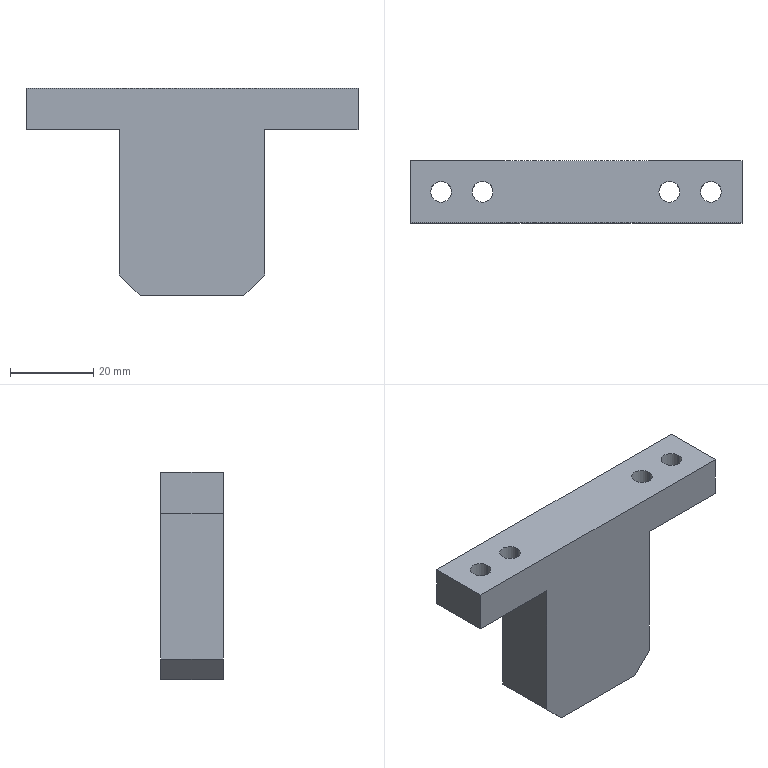Part | SolidWorks | features BaseBody 1 | 1 solid | 20 faces | box 80 x 15 x 50 mm | volume 31840 mm3 | plane 12 | cylinder 8 | commonest cylinder face diameters 5 x8
STEP:
#1=CARTESIAN_POINT('',(10.,7.5,-10.));
#2=VERTEX_POINT('',#1);
#3=CARTESIAN_POINT('',(5.,7.5,-10.));
#4=VERTEX_POINT('',#3);
#5=CARTESIAN_POINT('',(7.5,7.5,-10.));
#6=DIRECTION('',(0.,0.,-1.));
#7=DIRECTION('',(1.,0.,0.));
#8=AXIS2_PLACEMENT_3D('',#5,#6,#7);
#9=CIRCLE('',#8,2.5);
#10=EDGE_CURVE('',#2,#4,#9,.T.);
#11=ORIENTED_EDGE('',*,*,#10,.T.);
#12=CARTESIAN_POINT('',(5.,7.5,0.));
#13=VERTEX_POINT('',#12);
#14=CARTESIAN_POINT('',(5.,7.5,-10.));
#15=DIRECTION('',(0.,0.,1.));
#16=VECTOR('',#15,1000.);
#17=LINE('',#14,#16);
#18=EDGE_CURVE('',#4,#13,#17,.T.);
#19=ORIENTED_EDGE('',*,*,#18,.T.);
#20=CARTESIAN_POINT('',(10.,7.5,0.));
#21=VERTEX_POINT('',#20);
#22=CARTESIAN_POINT('',(7.5,7.5,0.));
#23=DIRECTION('',(0.,0.,1.));
#24=DIRECTION('',(1.,0.,0.));
#25=AXIS2_PLACEMENT_3D('',#22,#23,#24);
#26=CIRCLE('',#25,2.5);
#27=EDGE_CURVE('',#13,#21,#26,.T.);
#28=ORIENTED_EDGE('',*,*,#27,.T.);
#29=CARTESIAN_POINT('',(10.,7.5,-10.));
#30=DIRECTION('',(0.,0.,1.));
#31=VECTOR('',#30,1000.);
#32=LINE('',#29,#31);
#33=EDGE_CURVE('',#2,#21,#32,.T.);
#34=ORIENTED_EDGE('',*,*,#33,.F.);
#35=EDGE_LOOP('',(#11,#19,#28,#34));
#36=FACE_OUTER_BOUND('',#35,.T.);
#37=CARTESIAN_POINT('',(7.5,7.5,-10.));
#38=DIRECTION('',(0.,0.,1.));
#39=DIRECTION('',(1.,0.,0.));
#40=AXIS2_PLACEMENT_3D('',#37,#38,#39);
#41=CYLINDRICAL_SURFACE('',#40,2.5);
#42=ADVANCED_FACE('',(#36),#41,.F.);
#43=CARTESIAN_POINT('',(20.,7.5,-10.));
#44=VERTEX_POINT('',#43);
#45=CARTESIAN_POINT('',(15.,7.5,-10.));
#46=VERTEX_POINT('',#45);
#47=CARTESIAN_POINT('',(17.5,7.5,-10.));
#48=DIRECTION('',(0.,0.,-1.));
#49=DIRECTION('',(1.,0.,0.));
#50=AXIS2_PLACEMENT_3D('',#47,#48,#49);
#51=CIRCLE('',#50,2.5);
#52=EDGE_CURVE('',#44,#46,#51,.T.);
#53=ORIENTED_EDGE('',*,*,#52,.T.);
#54=CARTESIAN_POINT('',(15.,7.5,0.));
#55=VERTEX_POINT('',#54);
#56=CARTESIAN_POINT('',(15.,7.5,-10.));
#57=DIRECTION('',(0.,0.,1.));
#58=VECTOR('',#57,1000.);
#59=LINE('',#56,#58);
#60=EDGE_CURVE('',#46,#55,#59,.T.);
#61=ORIENTED_EDGE('',*,*,#60,.T.);
#62=CARTESIAN_POINT('',(20.,7.5,0.));
#63=VERTEX_POINT('',#62);
#64=CARTESIAN_POINT('',(17.5,7.5,0.));
#65=DIRECTION('',(0.,0.,1.));
#66=DIRECTION('',(1.,0.,0.));
#67=AXIS2_PLACEMENT_3D('',#64,#65,#66);
#68=CIRCLE('',#67,2.5);
#69=EDGE_CURVE('',#55,#63,#68,.T.);
#70=ORIENTED_EDGE('',*,*,#69,.T.);
#71=CARTESIAN_POINT('',(20.,7.5,-10.));
#72=DIRECTION('',(0.,0.,1.));
#73=VECTOR('',#72,1000.);
#74=LINE('',#71,#73);
#75=EDGE_CURVE('',#44,#63,#74,.T.);
#76=ORIENTED_EDGE('',*,*,#75,.F.);
#77=EDGE_LOOP('',(#53,#61,#70,#76));
#78=FACE_OUTER_BOUND('',#77,.T.);
#79=CARTESIAN_POINT('',(17.5,7.5,-10.));
#80=DIRECTION('',(0.,0.,1.));
#81=DIRECTION('',(1.,0.,0.));
#82=AXIS2_PLACEMENT_3D('',#79,#80,#81);
#83=CYLINDRICAL_SURFACE('',#82,2.5);
#84=ADVANCED_FACE('',(#78),#83,.F.);
#85=CARTESIAN_POINT('',(75.,7.5,-10.));
#86=VERTEX_POINT('',#85);
#87=CARTESIAN_POINT('',(70.,7.5,-10.));
#88=VERTEX_POINT('',#87);
#89=CARTESIAN_POINT('',(72.5,7.5,-10.));
#90=DIRECTION('',(0.,0.,-1.));
#91=DIRECTION('',(1.,0.,0.));
#92=AXIS2_PLACEMENT_3D('',#89,#90,#91);
#93=CIRCLE('',#92,2.5);
#94=EDGE_CURVE('',#86,#88,#93,.T.);
#95=ORIENTED_EDGE('',*,*,#94,.T.);
#96=CARTESIAN_POINT('',(70.,7.5,0.));
#97=VERTEX_POINT('',#96);
#98=CARTESIAN_POINT('',(70.,7.5,-10.));
#99=DIRECTION('',(0.,0.,1.));
#100=VECTOR('',#99,1000.);
#101=LINE('',#98,#100);
#102=EDGE_CURVE('',#88,#97,#101,.T.);
#103=ORIENTED_EDGE('',*,*,#102,.T.);
#104=CARTESIAN_POINT('',(75.,7.5,0.));
#105=VERTEX_POINT('',#104);
#106=CARTESIAN_POINT('',(72.5,7.5,0.));
#107=DIRECTION('',(0.,0.,1.));
#108=DIRECTION('',(1.,0.,0.));
#109=AXIS2_PLACEMENT_3D('',#106,#107,#108);
#110=CIRCLE('',#109,2.5);
#111=EDGE_CURVE('',#97,#105,#110,.T.);
#112=ORIENTED_EDGE('',*,*,#111,.T.);
#113=CARTESIAN_POINT('',(75.,7.5,-10.));
#114=DIRECTION('',(0.,0.,1.));
#115=VECTOR('',#114,1000.);
#116=LINE('',#113,#115);
#117=EDGE_CURVE('',#86,#105,#116,.T.);
#118=ORIENTED_EDGE('',*,*,#117,.F.);
#119=EDGE_LOOP('',(#95,#103,#112,#118));
#120=FACE_OUTER_BOUND('',#119,.T.);
#121=CARTESIAN_POINT('',(72.5,7.5,-10.));
#122=DIRECTION('',(0.,0.,1.));
#123=DIRECTION('',(1.,0.,0.));
#124=AXIS2_PLACEMENT_3D('',#121,#122,#123);
#125=CYLINDRICAL_SURFACE('',#124,2.5);
#126=ADVANCED_FACE('',(#120),#125,.F.);
#127=CARTESIAN_POINT('',(65.,7.5,-10.));
#128=VERTEX_POINT('',#127);
#129=CARTESIAN_POINT('',(60.,7.5,-10.));
#130=VERTEX_POINT('',#129);
#131=CARTESIAN_POINT('',(62.5,7.5,-10.));
#132=DIRECTION('',(0.,0.,-1.));
#133=DIRECTION('',(1.,0.,0.));
#134=AXIS2_PLACEMENT_3D('',#131,#132,#133);
#135=CIRCLE('',#134,2.5);
#136=EDGE_CURVE('',#128,#130,#135,.T.);
#137=ORIENTED_EDGE('',*,*,#136,.T.);
#138=CARTESIAN_POINT('',(60.,7.5,0.));
#139=VERTEX_POINT('',#138);
#140=CARTESIAN_POINT('',(60.,7.5,-10.));
#141=DIRECTION('',(0.,0.,1.));
#142=VECTOR('',#141,1000.);
#143=LINE('',#140,#142);
#144=EDGE_CURVE('',#130,#139,#143,.T.);
#145=ORIENTED_EDGE('',*,*,#144,.T.);
#146=CARTESIAN_POINT('',(65.,7.5,0.));
#147=VERTEX_POINT('',#146);
#148=CARTESIAN_POINT('',(62.5,7.5,0.));
#149=DIRECTION('',(0.,0.,1.));
#150=DIRECTION('',(1.,0.,0.));
#151=AXIS2_PLACEMENT_3D('',#148,#149,#150);
#152=CIRCLE('',#151,2.5);
#153=EDGE_CURVE('',#139,#147,#152,.T.);
#154=ORIENTED_EDGE('',*,*,#153,.T.);
#155=CARTESIAN_POINT('',(65.,7.5,-10.));
#156=DIRECTION('',(0.,0.,1.));
#157=VECTOR('',#156,1000.);
#158=LINE('',#155,#157);
#159=EDGE_CURVE('',#128,#147,#158,.T.);
#160=ORIENTED_EDGE('',*,*,#159,.F.);
#161=EDGE_LOOP('',(#137,#145,#154,#160));
#162=FACE_OUTER_BOUND('',#161,.T.);
#163=CARTESIAN_POINT('',(62.5,7.5,-10.));
#164=DIRECTION('',(0.,0.,1.));
#165=DIRECTION('',(1.,0.,0.));
#166=AXIS2_PLACEMENT_3D('',#163,#164,#165);
#167=CYLINDRICAL_SURFACE('',#166,2.5);
#168=ADVANCED_FACE('',(#162),#167,.F.);
#169=CARTESIAN_POINT('',(22.5,0.,-45.));
#170=VERTEX_POINT('',#169);
#171=CARTESIAN_POINT('',(22.5,0.,-10.));
#172=VERTEX_POINT('',#171);
#173=CARTESIAN_POINT('',(22.5,0.,0.));
#174=DIRECTION('',(0.,0.,1.));
#175=VECTOR('',#174,1000.);
#176=LINE('',#173,#175);
#177=EDGE_CURVE('',#170,#172,#176,.T.);
#178=ORIENTED_EDGE('',*,*,#177,.F.);
#179=CARTESIAN_POINT('',(27.5,0.,-50.));
#180=VERTEX_POINT('',#179);
#181=CARTESIAN_POINT('',(27.5,0.,-50.));
#182=DIRECTION('',(-0.7071,0.,0.7071));
#183=VECTOR('',#182,1000.);
#184=LINE('',#181,#183);
#185=EDGE_CURVE('',#180,#170,#184,.T.);
#186=ORIENTED_EDGE('',*,*,#185,.F.);
#187=CARTESIAN_POINT('',(52.5,0.,-50.));
#188=VERTEX_POINT('',#187);
#189=CARTESIAN_POINT('',(0.,0.,-50.));
#190=DIRECTION('',(-1.,0.,0.));
#191=VECTOR('',#190,1000.);
#192=LINE('',#189,#191);
#193=EDGE_CURVE('',#188,#180,#192,.T.);
#194=ORIENTED_EDGE('',*,*,#193,.F.);
#195=CARTESIAN_POINT('',(57.5,0.,-45.));
#196=VERTEX_POINT('',#195);
#197=CARTESIAN_POINT('',(57.5,0.,-45.));
#198=DIRECTION('',(-0.7071,0.,-0.7071));
#199=VECTOR('',#198,1000.);
#200=LINE('',#197,#199);
#201=EDGE_CURVE('',#196,#188,#200,.T.);
#202=ORIENTED_EDGE('',*,*,#201,.F.);
#203=CARTESIAN_POINT('',(57.5,0.,-10.));
#204=VERTEX_POINT('',#203);
#205=CARTESIAN_POINT('',(57.5,0.,0.));
#206=DIRECTION('',(0.,0.,-1.));
#207=VECTOR('',#206,1000.);
#208=LINE('',#205,#207);
#209=EDGE_CURVE('',#204,#196,#208,.T.);
#210=ORIENTED_EDGE('',*,*,#209,.F.);
#211=CARTESIAN_POINT('',(80.,0.,-10.));
#212=VERTEX_POINT('',#211);
#213=CARTESIAN_POINT('',(0.,0.,-10.));
#214=DIRECTION('',(-1.,0.,0.));
#215=VECTOR('',#214,1000.);
#216=LINE('',#213,#215);
#217=EDGE_CURVE('',#212,#204,#216,.T.);
#218=ORIENTED_EDGE('',*,*,#217,.F.);
#219=CARTESIAN_POINT('',(80.,0.,0.));
#220=VERTEX_POINT('',#219);
#221=CARTESIAN_POINT('',(80.,0.,0.));
#222=DIRECTION('',(0.,0.,-1.));
#223=VECTOR('',#222,1000.);
#224=LINE('',#221,#223);
#225=EDGE_CURVE('',#220,#212,#224,.T.);
#226=ORIENTED_EDGE('',*,*,#225,.F.);
#227=CARTESIAN_POINT('',(0.,0.,0.));
#228=VERTEX_POINT('',#227);
#229=CARTESIAN_POINT('',(0.,0.,0.));
#230=DIRECTION('',(1.,0.,0.));
#231=VECTOR('',#230,1000.);
#232=LINE('',#229,#231);
#233=EDGE_CURVE('',#228,#220,#232,.T.);
#234=ORIENTED_EDGE('',*,*,#233,.F.);
#235=CARTESIAN_POINT('',(0.,0.,-10.));
#236=VERTEX_POINT('',#235);
#237=CARTESIAN_POINT('',(0.,0.,0.));
#238=DIRECTION('',(0.,0.,1.));
#239=VECTOR('',#238,1000.);
#240=LINE('',#237,#239);
#241=EDGE_CURVE('',#236,#228,#240,.T.);
#242=ORIENTED_EDGE('',*,*,#241,.F.);
#243=CARTESIAN_POINT('',(0.,0.,-10.));
#244=DIRECTION('',(-1.,0.,0.));
#245=VECTOR('',#244,1000.);
#246=LINE('',#243,#245);
#247=EDGE_CURVE('',#172,#236,#246,.T.);
#248=ORIENTED_EDGE('',*,*,#247,.F.);
#249=EDGE_LOOP('',(#178,#186,#194,#202,#210,#218,#226,#234,#242,#248));
#250=FACE_OUTER_BOUND('',#249,.T.);
#251=CARTESIAN_POINT('',(0.,0.,0.));
#252=DIRECTION('',(0.,1.,0.));
#253=DIRECTION('',(0.,0.,1.));
#254=AXIS2_PLACEMENT_3D('',#251,#252,#253);
#255=PLANE('',#254);
#256=ADVANCED_FACE('',(#250),#255,.F.);
#257=CARTESIAN_POINT('',(22.5,15.,-10.));
#258=VERTEX_POINT('',#257);
#259=CARTESIAN_POINT('',(0.,15.,-10.));
#260=VERTEX_POINT('',#259);
#261=CARTESIAN_POINT('',(22.5,15.,-10.));
#262=DIRECTION('',(-1.,0.,0.));
#263=VECTOR('',#262,1000.);
#264=LINE('',#261,#263);
#265=EDGE_CURVE('',#258,#260,#264,.T.);
#266=ORIENTED_EDGE('',*,*,#265,.F.);
#267=CARTESIAN_POINT('',(22.5,16.5,-10.));
#268=DIRECTION('',(0.,1.,0.));
#269=VECTOR('',#268,1000.);
#270=LINE('',#267,#269);
#271=EDGE_CURVE('',#172,#258,#270,.T.);
#272=ORIENTED_EDGE('',*,*,#271,.F.);
#273=ORIENTED_EDGE('',*,*,#247,.T.);
#274=CARTESIAN_POINT('',(0.,16.5,-10.));
#275=DIRECTION('',(0.,-1.,0.));
#276=VECTOR('',#275,1000.);
#277=LINE('',#274,#276);
#278=EDGE_CURVE('',#260,#236,#277,.T.);
#279=ORIENTED_EDGE('',*,*,#278,.F.);
#280=EDGE_LOOP('',(#266,#272,#273,#279));
#281=FACE_OUTER_BOUND('',#280,.T.);
#282=ORIENTED_EDGE('',*,*,#10,.F.);
#283=CARTESIAN_POINT('',(7.5,7.5,-10.));
#284=DIRECTION('',(0.,0.,-1.));
#285=DIRECTION('',(1.,0.,0.));
#286=AXIS2_PLACEMENT_3D('',#283,#284,#285);
#287=CIRCLE('',#286,2.5);
#288=EDGE_CURVE('',#4,#2,#287,.T.);
#289=ORIENTED_EDGE('',*,*,#288,.F.);
#290=EDGE_LOOP('',(#282,#289));
#291=FACE_BOUND('',#290,.T.);
#292=ORIENTED_EDGE('',*,*,#52,.F.);
#293=CARTESIAN_POINT('',(17.5,7.5,-10.));
#294=DIRECTION('',(0.,0.,-1.));
#295=DIRECTION('',(1.,0.,0.));
#296=AXIS2_PLACEMENT_3D('',#293,#294,#295);
#297=CIRCLE('',#296,2.5);
#298=EDGE_CURVE('',#46,#44,#297,.T.);
#299=ORIENTED_EDGE('',*,*,#298,.F.);
#300=EDGE_LOOP('',(#292,#299));
#301=FACE_BOUND('',#300,.T.);
#302=CARTESIAN_POINT('',(22.5,16.5,-10.));
#303=DIRECTION('',(0.,0.,1.));
#304=DIRECTION('',(1.,0.,0.));
#305=AXIS2_PLACEMENT_3D('',#302,#303,#304);
#306=PLANE('',#305);
#307=ADVANCED_FACE('',(#281,#291,#301),#306,.F.);
#308=CARTESIAN_POINT('',(22.5,15.,-45.));
#309=VERTEX_POINT('',#308);
#310=CARTESIAN_POINT('',(22.5,15.,-45.));
#311=DIRECTION('',(0.,0.,1.));
#312=VECTOR('',#311,1000.);
#313=LINE('',#310,#312);
#314=EDGE_CURVE('',#309,#258,#313,.T.);
#315=ORIENTED_EDGE('',*,*,#314,.F.);
#316=CARTESIAN_POINT('',(22.5,16.5,-45.));
#317=DIRECTION('',(0.,1.,0.));
#318=VECTOR('',#317,1000.);
#319=LINE('',#316,#318);
#320=EDGE_CURVE('',#170,#309,#319,.T.);
#321=ORIENTED_EDGE('',*,*,#320,.F.);
#322=ORIENTED_EDGE('',*,*,#177,.T.);
#323=ORIENTED_EDGE('',*,*,#271,.T.);
#324=EDGE_LOOP('',(#315,#321,#322,#323));
#325=FACE_OUTER_BOUND('',#324,.T.);
#326=CARTESIAN_POINT('',(22.5,16.5,-45.));
#327=DIRECTION('',(1.,0.,0.));
#328=DIRECTION('',(0.,0.,-1.));
#329=AXIS2_PLACEMENT_3D('',#326,#327,#328);
#330=PLANE('',#329);
#331=ADVANCED_FACE('',(#325),#330,.F.);
#332=CARTESIAN_POINT('',(27.5,15.,-50.));
#333=VERTEX_POINT('',#332);
#334=CARTESIAN_POINT('',(27.5,15.,-50.));
#335=DIRECTION('',(-0.7071,0.,0.7071));
#336=VECTOR('',#335,1000.);
#337=LINE('',#334,#336);
#338=EDGE_CURVE('',#333,#309,#337,.T.);
#339=ORIENTED_EDGE('',*,*,#338,.F.);
#340=CARTESIAN_POINT('',(27.5,16.5,-50.));
#341=DIRECTION('',(0.,1.,0.));
#342=VECTOR('',#341,1000.);
#343=LINE('',#340,#342);
#344=EDGE_CURVE('',#180,#333,#343,.T.);
#345=ORIENTED_EDGE('',*,*,#344,.F.);
#346=ORIENTED_EDGE('',*,*,#185,.T.);
#347=ORIENTED_EDGE('',*,*,#320,.T.);
#348=EDGE_LOOP('',(#339,#345,#346,#347));
#349=FACE_OUTER_BOUND('',#348,.T.);
#350=CARTESIAN_POINT('',(27.5,16.5,-50.));
#351=DIRECTION('',(0.7071,0.,0.7071));
#352=DIRECTION('',(0.7071,0.,-0.7071));
#353=AXIS2_PLACEMENT_3D('',#350,#351,#352);
#354=PLANE('',#353);
#355=ADVANCED_FACE('',(#349),#354,.F.);
#356=CARTESIAN_POINT('',(52.5,15.,-50.));
#357=VERTEX_POINT('',#356);
#358=CARTESIAN_POINT('',(80.,15.,-50.));
#359=DIRECTION('',(-1.,0.,0.));
#360=VECTOR('',#359,1000.);
#361=LINE('',#358,#360);
#362=EDGE_CURVE('',#357,#333,#361,.T.);
#363=ORIENTED_EDGE('',*,*,#362,.F.);
#364=CARTESIAN_POINT('',(52.5,15.,-50.));
#365=DIRECTION('',(0.,1.,0.));
#366=VECTOR('',#365,1000.);
#367=LINE('',#364,#366);
#368=EDGE_CURVE('',#188,#357,#367,.T.);
#369=ORIENTED_EDGE('',*,*,#368,.F.);
#370=ORIENTED_EDGE('',*,*,#193,.T.);
#371=ORIENTED_EDGE('',*,*,#344,.T.);
#372=EDGE_LOOP('',(#363,#369,#370,#371));
#373=FACE_OUTER_BOUND('',#372,.T.);
#374=CARTESIAN_POINT('',(80.,15.,-50.));
#375=DIRECTION('',(0.,0.,1.));
#376=DIRECTION('',(1.,0.,0.));
#377=AXIS2_PLACEMENT_3D('',#374,#375,#376);
#378=PLANE('',#377);
#379=ADVANCED_FACE('',(#373),#378,.F.);
#380=CARTESIAN_POINT('',(57.5,15.,-45.));
#381=VERTEX_POINT('',#380);
#382=CARTESIAN_POINT('',(57.5,15.,-45.));
#383=DIRECTION('',(-0.7071,0.,-0.7071));
#384=VECTOR('',#383,1000.);
#385=LINE('',#382,#384);
#386=EDGE_CURVE('',#381,#357,#385,.T.);
#387=ORIENTED_EDGE('',*,*,#386,.F.);
#388=CARTESIAN_POINT('',(57.5,16.5,-45.));
#389=DIRECTION('',(0.,1.,0.));
#390=VECTOR('',#389,1000.);
#391=LINE('',#388,#390);
#392=EDGE_CURVE('',#196,#381,#391,.T.);
#393=ORIENTED_EDGE('',*,*,#392,.F.);
#394=ORIENTED_EDGE('',*,*,#201,.T.);
#395=ORIENTED_EDGE('',*,*,#368,.T.);
#396=EDGE_LOOP('',(#387,#393,#394,#395));
#397=FACE_OUTER_BOUND('',#396,.T.);
#398=CARTESIAN_POINT('',(57.5,16.5,-45.));
#399=DIRECTION('',(-0.7071,0.,0.7071));
#400=DIRECTION('',(0.7071,0.,0.7071));
#401=AXIS2_PLACEMENT_3D('',#398,#399,#400);
#402=PLANE('',#401);
#403=ADVANCED_FACE('',(#397),#402,.F.);
#404=CARTESIAN_POINT('',(57.5,15.,-10.));
#405=VERTEX_POINT('',#404);
#406=CARTESIAN_POINT('',(57.5,15.,-10.));
#407=DIRECTION('',(0.,0.,-1.));
#408=VECTOR('',#407,1000.);
#409=LINE('',#406,#408);
#410=EDGE_CURVE('',#405,#381,#409,.T.);
#411=ORIENTED_EDGE('',*,*,#410,.F.);
#412=CARTESIAN_POINT('',(57.5,16.5,-10.));
#413=DIRECTION('',(0.,1.,0.));
#414=VECTOR('',#413,1000.);
#415=LINE('',#412,#414);
#416=EDGE_CURVE('',#204,#405,#415,.T.);
#417=ORIENTED_EDGE('',*,*,#416,.F.);
#418=ORIENTED_EDGE('',*,*,#209,.T.);
#419=ORIENTED_EDGE('',*,*,#392,.T.);
#420=EDGE_LOOP('',(#411,#417,#418,#419));
#421=FACE_OUTER_BOUND('',#420,.T.);
#422=CARTESIAN_POINT('',(57.5,16.5,-10.));
#423=DIRECTION('',(-1.,0.,0.));
#424=DIRECTION('',(0.,0.,1.));
#425=AXIS2_PLACEMENT_3D('',#422,#423,#424);
#426=PLANE('',#425);
#427=ADVANCED_FACE('',(#421),#426,.F.);
#428=CARTESIAN_POINT('',(80.,15.,-10.));
#429=VERTEX_POINT('',#428);
#430=CARTESIAN_POINT('',(80.,15.,-10.));
#431=DIRECTION('',(-1.,0.,0.));
#432=VECTOR('',#431,1000.);
#433=LINE('',#430,#432);
#434=EDGE_CURVE('',#429,#405,#433,.T.);
#435=ORIENTED_EDGE('',*,*,#434,.F.);
#436=CARTESIAN_POINT('',(80.,16.5,-10.));
#437=DIRECTION('',(0.,1.,0.));
#438=VECTOR('',#437,1000.);
#439=LINE('',#436,#438);
#440=EDGE_CURVE('',#212,#429,#439,.T.);
#441=ORIENTED_EDGE('',*,*,#440,.F.);
#442=ORIENTED_EDGE('',*,*,#217,.T.);
#443=ORIENTED_EDGE('',*,*,#416,.T.);
#444=EDGE_LOOP('',(#435,#441,#442,#443));
#445=FACE_OUTER_BOUND('',#444,.T.);
#446=ORIENTED_EDGE('',*,*,#94,.F.);
#447=CARTESIAN_POINT('',(72.5,7.5,-10.));
#448=DIRECTION('',(0.,0.,-1.));
#449=DIRECTION('',(1.,0.,0.));
#450=AXIS2_PLACEMENT_3D('',#447,#448,#449);
#451=CIRCLE('',#450,2.5);
#452=EDGE_CURVE('',#88,#86,#451,.T.);
#453=ORIENTED_EDGE('',*,*,#452,.F.);
#454=EDGE_LOOP('',(#446,#453));
#455=FACE_BOUND('',#454,.T.);
#456=ORIENTED_EDGE('',*,*,#136,.F.);
#457=CARTESIAN_POINT('',(62.5,7.5,-10.));
#458=DIRECTION('',(0.,0.,-1.));
#459=DIRECTION('',(1.,0.,0.));
#460=AXIS2_PLACEMENT_3D('',#457,#458,#459);
#461=CIRCLE('',#460,2.5);
#462=EDGE_CURVE('',#130,#128,#461,.T.);
#463=ORIENTED_EDGE('',*,*,#462,.F.);
#464=EDGE_LOOP('',(#456,#463));
#465=FACE_BOUND('',#464,.T.);
#466=CARTESIAN_POINT('',(80.,16.5,-10.));
#467=DIRECTION('',(0.,0.,1.));
#468=DIRECTION('',(1.,0.,0.));
#469=AXIS2_PLACEMENT_3D('',#466,#467,#468);
#470=PLANE('',#469);
#471=ADVANCED_FACE('',(#445,#455,#465),#470,.F.);
#472=CARTESIAN_POINT('',(80.,15.,0.));
#473=VERTEX_POINT('',#472);
#474=CARTESIAN_POINT('',(80.,15.,0.));
#475=DIRECTION('',(0.,0.,-1.));
#476=VECTOR('',#475,1000.);
#477=LINE('',#474,#476);
#478=EDGE_CURVE('',#473,#429,#477,.T.);
#479=ORIENTED_EDGE('',*,*,#478,.F.);
#480=CARTESIAN_POINT('',(80.,15.,0.));
#481=DIRECTION('',(0.,1.,0.));
#482=VECTOR('',#481,1000.);
#483=LINE('',#480,#482);
#484=EDGE_CURVE('',#220,#473,#483,.T.);
#485=ORIENTED_EDGE('',*,*,#484,.F.);
#486=ORIENTED_EDGE('',*,*,#225,.T.);
#487=ORIENTED_EDGE('',*,*,#440,.T.);
#488=EDGE_LOOP('',(#479,#485,#486,#487));
#489=FACE_OUTER_BOUND('',#488,.T.);
#490=CARTESIAN_POINT('',(80.,15.,0.));
#491=DIRECTION('',(-1.,0.,0.));
#492=DIRECTION('',(0.,0.,1.));
#493=AXIS2_PLACEMENT_3D('',#490,#491,#492);
#494=PLANE('',#493);
#495=ADVANCED_FACE('',(#489),#494,.F.);
#496=ORIENTED_EDGE('',*,*,#484,.T.);
#497=CARTESIAN_POINT('',(0.,15.,0.));
#498=VERTEX_POINT('',#497);
#499=CARTESIAN_POINT('',(0.,15.,0.));
#500=DIRECTION('',(1.,0.,0.));
#501=VECTOR('',#500,1000.);
#502=LINE('',#499,#501);
#503=EDGE_CURVE('',#498,#473,#502,.T.);
#504=ORIENTED_EDGE('',*,*,#503,.F.);
#505=CARTESIAN_POINT('',(0.,15.,0.));
#506=DIRECTION('',(0.,1.,0.));
#507=VECTOR('',#506,1000.);
#508=LINE('',#505,#507);
#509=EDGE_CURVE('',#228,#498,#508,.T.);
#510=ORIENTED_EDGE('',*,*,#509,.F.);
#511=ORIENTED_EDGE('',*,*,#233,.T.);
#512=EDGE_LOOP('',(#496,#504,#510,#511));
#513=FACE_OUTER_BOUND('',#512,.T.);
#514=CARTESIAN_POINT('',(7.5,7.5,0.));
#515=DIRECTION('',(0.,0.,1.));
#516=DIRECTION('',(1.,0.,0.));
#517=AXIS2_PLACEMENT_3D('',#514,#515,#516);
#518=CIRCLE('',#517,2.5);
#519=EDGE_CURVE('',#21,#13,#518,.T.);
#520=ORIENTED_EDGE('',*,*,#519,.F.);
#521=ORIENTED_EDGE('',*,*,#27,.F.);
#522=EDGE_LOOP('',(#520,#521));
#523=FACE_BOUND('',#522,.T.);
#524=CARTESIAN_POINT('',(17.5,7.5,0.));
#525=DIRECTION('',(0.,0.,1.));
#526=DIRECTION('',(1.,0.,0.));
#527=AXIS2_PLACEMENT_3D('',#524,#525,#526);
#528=CIRCLE('',#527,2.5);
#529=EDGE_CURVE('',#63,#55,#528,.T.);
#530=ORIENTED_EDGE('',*,*,#529,.F.);
#531=ORIENTED_EDGE('',*,*,#69,.F.);
#532=EDGE_LOOP('',(#530,#531));
#533=FACE_BOUND('',#532,.T.);
#534=CARTESIAN_POINT('',(72.5,7.5,0.));
#535=DIRECTION('',(0.,0.,1.));
#536=DIRECTION('',(1.,0.,0.));
#537=AXIS2_PLACEMENT_3D('',#534,#535,#536);
#538=CIRCLE('',#537,2.5);
#539=EDGE_CURVE('',#105,#97,#538,.T.);
#540=ORIENTED_EDGE('',*,*,#539,.F.);
#541=ORIENTED_EDGE('',*,*,#111,.F.);
#542=EDGE_LOOP('',(#540,#541));
#543=FACE_BOUND('',#542,.T.);
#544=CARTESIAN_POINT('',(62.5,7.5,0.));
#545=DIRECTION('',(0.,0.,1.));
#546=DIRECTION('',(1.,0.,0.));
#547=AXIS2_PLACEMENT_3D('',#544,#545,#546);
#548=CIRCLE('',#547,2.5);
#549=EDGE_CURVE('',#147,#139,#548,.T.);
#550=ORIENTED_EDGE('',*,*,#549,.F.);
#551=ORIENTED_EDGE('',*,*,#153,.F.);
#552=EDGE_LOOP('',(#550,#551));
#553=FACE_BOUND('',#552,.T.);
#554=CARTESIAN_POINT('',(0.,15.,0.));
#555=DIRECTION('',(0.,0.,-1.));
#556=DIRECTION('',(-1.,0.,0.));
#557=AXIS2_PLACEMENT_3D('',#554,#555,#556);
#558=PLANE('',#557);
#559=ADVANCED_FACE('',(#513,#523,#533,#543,#553),#558,.F.);
#560=ORIENTED_EDGE('',*,*,#278,.T.);
#561=ORIENTED_EDGE('',*,*,#241,.T.);
#562=ORIENTED_EDGE('',*,*,#509,.T.);
#563=CARTESIAN_POINT('',(0.,15.,-50.));
#564=DIRECTION('',(0.,0.,1.));
#565=VECTOR('',#564,1000.);
#566=LINE('',#563,#565);
#567=EDGE_CURVE('',#260,#498,#566,.T.);
#568=ORIENTED_EDGE('',*,*,#567,.F.);
#569=EDGE_LOOP('',(#560,#561,#562,#568));
#570=FACE_OUTER_BOUND('',#569,.T.);
#571=CARTESIAN_POINT('',(0.,15.,-50.));
#572=DIRECTION('',(1.,0.,0.));
#573=DIRECTION('',(0.,0.,-1.));
#574=AXIS2_PLACEMENT_3D('',#571,#572,#573);
#575=PLANE('',#574);
#576=ADVANCED_FACE('',(#570),#575,.F.);
#577=ORIENTED_EDGE('',*,*,#386,.T.);
#578=ORIENTED_EDGE('',*,*,#362,.T.);
#579=ORIENTED_EDGE('',*,*,#338,.T.);
#580=ORIENTED_EDGE('',*,*,#314,.T.);
#581=ORIENTED_EDGE('',*,*,#265,.T.);
#582=ORIENTED_EDGE('',*,*,#567,.T.);
#583=ORIENTED_EDGE('',*,*,#503,.T.);
#584=ORIENTED_EDGE('',*,*,#478,.T.);
#585=ORIENTED_EDGE('',*,*,#434,.T.);
#586=ORIENTED_EDGE('',*,*,#410,.T.);
#587=EDGE_LOOP('',(#577,#578,#579,#580,#581,#582,#583,#584,#585,#586));
#588=FACE_OUTER_BOUND('',#587,.T.);
#589=CARTESIAN_POINT('',(0.,15.,0.));
#590=DIRECTION('',(0.,1.,0.));
#591=DIRECTION('',(0.,0.,1.));
#592=AXIS2_PLACEMENT_3D('',#589,#590,#591);
#593=PLANE('',#592);
#594=ADVANCED_FACE('',(#588),#593,.T.);
#595=ORIENTED_EDGE('',*,*,#18,.F.);
#596=ORIENTED_EDGE('',*,*,#288,.T.);
#597=ORIENTED_EDGE('',*,*,#33,.T.);
#598=ORIENTED_EDGE('',*,*,#519,.T.);
#599=EDGE_LOOP('',(#595,#596,#597,#598));
#600=FACE_OUTER_BOUND('',#599,.T.);
#601=CARTESIAN_POINT('',(7.5,7.5,-10.));
#602=DIRECTION('',(0.,0.,1.));
#603=DIRECTION('',(1.,0.,0.));
#604=AXIS2_PLACEMENT_3D('',#601,#602,#603);
#605=CYLINDRICAL_SURFACE('',#604,2.5);
#606=ADVANCED_FACE('',(#600),#605,.F.);
#607=ORIENTED_EDGE('',*,*,#60,.F.);
#608=ORIENTED_EDGE('',*,*,#298,.T.);
#609=ORIENTED_EDGE('',*,*,#75,.T.);
#610=ORIENTED_EDGE('',*,*,#529,.T.);
#611=EDGE_LOOP('',(#607,#608,#609,#610));
#612=FACE_OUTER_BOUND('',#611,.T.);
#613=CARTESIAN_POINT('',(17.5,7.5,-10.));
#614=DIRECTION('',(0.,0.,1.));
#615=DIRECTION('',(1.,0.,0.));
#616=AXIS2_PLACEMENT_3D('',#613,#614,#615);
#617=CYLINDRICAL_SURFACE('',#616,2.5);
#618=ADVANCED_FACE('',(#612),#617,.F.);
#619=ORIENTED_EDGE('',*,*,#102,.F.);
#620=ORIENTED_EDGE('',*,*,#452,.T.);
#621=ORIENTED_EDGE('',*,*,#117,.T.);
#622=ORIENTED_EDGE('',*,*,#539,.T.);
#623=EDGE_LOOP('',(#619,#620,#621,#622));
#624=FACE_OUTER_BOUND('',#623,.T.);
#625=CARTESIAN_POINT('',(72.5,7.5,-10.));
#626=DIRECTION('',(0.,0.,1.));
#627=DIRECTION('',(1.,0.,0.));
#628=AXIS2_PLACEMENT_3D('',#625,#626,#627);
#629=CYLINDRICAL_SURFACE('',#628,2.5);
#630=ADVANCED_FACE('',(#624),#629,.F.);
#631=ORIENTED_EDGE('',*,*,#144,.F.);
#632=ORIENTED_EDGE('',*,*,#462,.T.);
#633=ORIENTED_EDGE('',*,*,#159,.T.);
#634=ORIENTED_EDGE('',*,*,#549,.T.);
#635=EDGE_LOOP('',(#631,#632,#633,#634));
#636=FACE_OUTER_BOUND('',#635,.T.);
#637=CARTESIAN_POINT('',(62.5,7.5,-10.));
#638=DIRECTION('',(0.,0.,1.));
#639=DIRECTION('',(1.,0.,0.));
#640=AXIS2_PLACEMENT_3D('',#637,#638,#639);
#641=CYLINDRICAL_SURFACE('',#640,2.5);
#642=ADVANCED_FACE('',(#636),#641,.F.);
#643=CLOSED_SHELL('',(#42,#84,#126,#168,#256,#307,#331,#355,#379,#403,#427,#471,#495,#559,#576,#594,#606,#618,#630,#642));
#644=MANIFOLD_SOLID_BREP('',#643);
#645=CARTESIAN_POINT('',(0.,0.,0.));
#646=DIRECTION('',(0.,0.,1.));
#647=DIRECTION('',(1.,0.,0.));
#648=AXIS2_PLACEMENT_3D('',#645,#646,#647);
#649=(LENGTH_UNIT()NAMED_UNIT(*)SI_UNIT(.MILLI.,.METRE.));
#650=UNCERTAINTY_MEASURE_WITH_UNIT(LENGTH_MEASURE(0.00001),#649,'','');
#651=(NAMED_UNIT(*)PLANE_ANGLE_UNIT()SI_UNIT($,.RADIAN.));
#652=(NAMED_UNIT(*)SI_UNIT($,.STERADIAN.)SOLID_ANGLE_UNIT());
#653=(GEOMETRIC_REPRESENTATION_CONTEXT(3)GLOBAL_UNCERTAINTY_ASSIGNED_CONTEXT((#650))GLOBAL_UNIT_ASSIGNED_CONTEXT((#649,#651,#652))REPRESENTATION_CONTEXT('',''));
#654=ADVANCED_BREP_SHAPE_REPRESENTATION('',(#644,#648),#653);